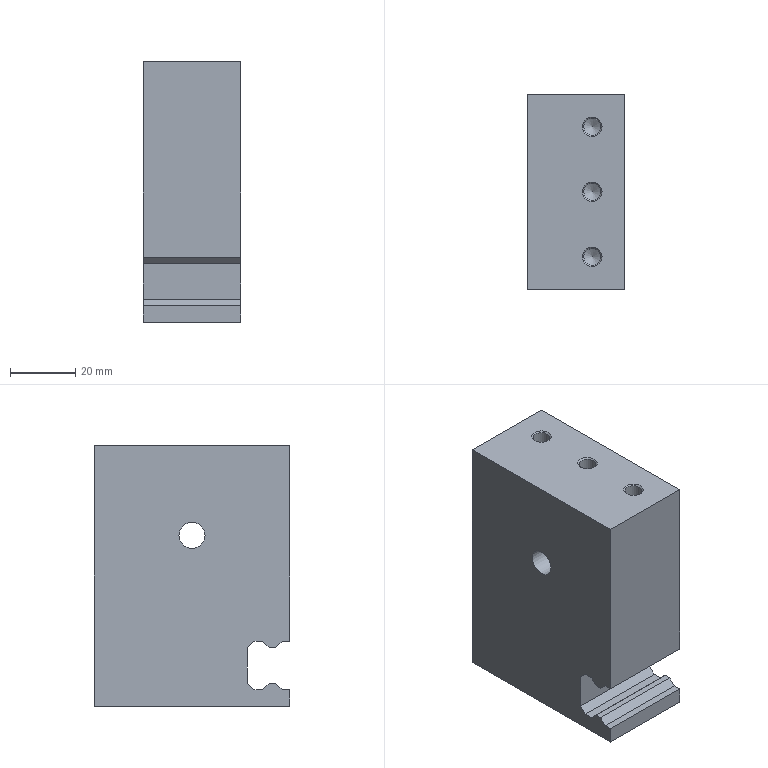Part | NX | features CBORE_HOLE 8, DATUM_CSYS 6, SYMBOLIC_THREAD 6, SIMPLE HOLE 5, SKETCH 5, HOLE PACKAGE 3, EXTRUDE 2, SUBTRACT 1 | 1 solid | 36 faces | box 30 x 60 x 80 mm | volume 135184 mm3 | plane 20 | cone 10 | cylinder 6 | commonest cylinder face diameters 5.2 x5 8 x1
STEP:
#1=CARTESIAN_POINT('',(15.,-2.3,7.5));
#2=VERTEX_POINT('',#1);
#3=CARTESIAN_POINT('',(-15.,-2.3,7.5));
#4=VERTEX_POINT('',#3);
#5=CARTESIAN_POINT('',(15.,-2.3,7.5));
#6=DIRECTION('',(-1.,0.,0.));
#7=VECTOR('',#6,1000.);
#8=LINE('',#5,#7);
#9=EDGE_CURVE('',#2,#4,#8,.T.);
#10=ORIENTED_EDGE('',*,*,#9,.F.);
#11=CARTESIAN_POINT('',(15.,-2.3,67.5));
#12=VERTEX_POINT('',#11);
#13=CARTESIAN_POINT('',(15.,-2.3,67.5));
#14=DIRECTION('',(0.,0.,-1.));
#15=VECTOR('',#14,1000.);
#16=LINE('',#13,#15);
#17=EDGE_CURVE('',#12,#2,#16,.T.);
#18=ORIENTED_EDGE('',*,*,#17,.F.);
#19=CARTESIAN_POINT('',(-15.,-2.3,67.5));
#20=VERTEX_POINT('',#19);
#21=CARTESIAN_POINT('',(15.,-2.3,67.5));
#22=DIRECTION('',(-1.,0.,0.));
#23=VECTOR('',#22,1000.);
#24=LINE('',#21,#23);
#25=EDGE_CURVE('',#12,#20,#24,.T.);
#26=ORIENTED_EDGE('',*,*,#25,.T.);
#27=CARTESIAN_POINT('',(-15.,-2.3,67.5));
#28=DIRECTION('',(0.,0.,-1.));
#29=VECTOR('',#28,1000.);
#30=LINE('',#27,#29);
#31=EDGE_CURVE('',#20,#4,#30,.T.);
#32=ORIENTED_EDGE('',*,*,#31,.T.);
#33=EDGE_LOOP('',(#10,#18,#26,#32));
#34=FACE_BOUND('',#33,.T.);
#35=CARTESIAN_POINT('',(15.,-2.3,67.5));
#36=DIRECTION('',(0.,1.,0.));
#37=DIRECTION('',(0.,0.,1.));
#38=AXIS2_PLACEMENT_3D('',#35,#36,#37);
#39=PLANE('',#38);
#40=ADVANCED_FACE('',(#34),#39,.F.);
#41=CARTESIAN_POINT('',(-15.,-2.3,-7.5));
#42=VERTEX_POINT('',#41);
#43=CARTESIAN_POINT('',(15.,-2.3,-7.5));
#44=VERTEX_POINT('',#43);
#45=CARTESIAN_POINT('',(15.,-2.3,-7.5));
#46=DIRECTION('',(1.,0.,0.));
#47=VECTOR('',#46,1000.);
#48=LINE('',#45,#47);
#49=EDGE_CURVE('',#42,#44,#48,.T.);
#50=ORIENTED_EDGE('',*,*,#49,.F.);
#51=CARTESIAN_POINT('',(-15.,-2.3,-12.5));
#52=VERTEX_POINT('',#51);
#53=CARTESIAN_POINT('',(-15.,-2.3,67.5));
#54=DIRECTION('',(0.,0.,-1.));
#55=VECTOR('',#54,1000.);
#56=LINE('',#53,#55);
#57=EDGE_CURVE('',#42,#52,#56,.T.);
#58=ORIENTED_EDGE('',*,*,#57,.T.);
#59=CARTESIAN_POINT('',(15.,-2.3,-12.5));
#60=VERTEX_POINT('',#59);
#61=CARTESIAN_POINT('',(15.,-2.3,-12.5));
#62=DIRECTION('',(-1.,0.,0.));
#63=VECTOR('',#62,1000.);
#64=LINE('',#61,#63);
#65=EDGE_CURVE('',#60,#52,#64,.T.);
#66=ORIENTED_EDGE('',*,*,#65,.F.);
#67=CARTESIAN_POINT('',(15.,-2.3,67.5));
#68=DIRECTION('',(0.,0.,-1.));
#69=VECTOR('',#68,1000.);
#70=LINE('',#67,#69);
#71=EDGE_CURVE('',#44,#60,#70,.T.);
#72=ORIENTED_EDGE('',*,*,#71,.F.);
#73=EDGE_LOOP('',(#50,#58,#66,#72));
#74=FACE_BOUND('',#73,.T.);
#75=CARTESIAN_POINT('',(15.,-2.3,67.5));
#76=DIRECTION('',(0.,1.,0.));
#77=DIRECTION('',(0.,0.,1.));
#78=AXIS2_PLACEMENT_3D('',#75,#76,#77);
#79=PLANE('',#78);
#80=ADVANCED_FACE('',(#74),#79,.F.);
#81=CARTESIAN_POINT('',(15.,31.7,40.));
#82=VERTEX_POINT('',#81);
#83=CARTESIAN_POINT('',(15.,27.7,40.));
#84=DIRECTION('',(1.,0.,0.));
#85=DIRECTION('',(0.,1.,0.));
#86=AXIS2_PLACEMENT_3D('',#83,#84,#85);
#87=CIRCLE('',#86,4.);
#88=EDGE_CURVE('',#82,#82,#87,.T.);
#89=ORIENTED_EDGE('',*,*,#88,.F.);
#90=EDGE_LOOP('',(#89));
#91=FACE_BOUND('',#90,.T.);
#92=ORIENTED_EDGE('',*,*,#17,.T.);
#93=CARTESIAN_POINT('',(15.,0.,7.5));
#94=VERTEX_POINT('',#93);
#95=CARTESIAN_POINT('',(15.,27.7,7.5));
#96=DIRECTION('',(0.,1.,0.));
#97=VECTOR('',#96,1000.);
#98=LINE('',#95,#97);
#99=EDGE_CURVE('',#2,#94,#98,.T.);
#100=ORIENTED_EDGE('',*,*,#99,.T.);
#101=CARTESIAN_POINT('',(15.,2.,5.5));
#102=VERTEX_POINT('',#101);
#103=CARTESIAN_POINT('',(15.,-2.4,9.9));
#104=DIRECTION('',(0.,0.7071,-0.7071));
#105=VECTOR('',#104,1000.);
#106=LINE('',#103,#105);
#107=EDGE_CURVE('',#94,#102,#106,.T.);
#108=ORIENTED_EDGE('',*,*,#107,.T.);
#109=CARTESIAN_POINT('',(15.,4.,5.5));
#110=VERTEX_POINT('',#109);
#111=CARTESIAN_POINT('',(15.,27.7,5.5));
#112=DIRECTION('',(0.,1.,0.));
#113=VECTOR('',#112,1000.);
#114=LINE('',#111,#113);
#115=EDGE_CURVE('',#102,#110,#114,.T.);
#116=ORIENTED_EDGE('',*,*,#115,.T.);
#117=CARTESIAN_POINT('',(15.,6.,7.5));
#118=VERTEX_POINT('',#117);
#119=CARTESIAN_POINT('',(15.,33.1,34.6));
#120=DIRECTION('',(0.,0.7071,0.7071));
#121=VECTOR('',#120,1000.);
#122=LINE('',#119,#121);
#123=EDGE_CURVE('',#110,#118,#122,.T.);
#124=ORIENTED_EDGE('',*,*,#123,.T.);
#125=CARTESIAN_POINT('',(15.,8.7,7.5));
#126=VERTEX_POINT('',#125);
#127=CARTESIAN_POINT('',(15.,27.7,7.5));
#128=DIRECTION('',(0.,1.,0.));
#129=VECTOR('',#128,1000.);
#130=LINE('',#127,#129);
#131=EDGE_CURVE('',#118,#126,#130,.T.);
#132=ORIENTED_EDGE('',*,*,#131,.T.);
#133=CARTESIAN_POINT('',(15.,10.7,5.5));
#134=VERTEX_POINT('',#133);
#135=CARTESIAN_POINT('',(15.,1.95,14.25));
#136=DIRECTION('',(0.,0.7071,-0.7071));
#137=VECTOR('',#136,1000.);
#138=LINE('',#135,#137);
#139=EDGE_CURVE('',#126,#134,#138,.T.);
#140=ORIENTED_EDGE('',*,*,#139,.T.);
#141=CARTESIAN_POINT('',(15.,10.7,-5.5));
#142=VERTEX_POINT('',#141);
#143=CARTESIAN_POINT('',(15.,10.7,40.));
#144=DIRECTION('',(0.,0.,-1.));
#145=VECTOR('',#144,1000.);
#146=LINE('',#143,#145);
#147=EDGE_CURVE('',#134,#142,#146,.T.);
#148=ORIENTED_EDGE('',*,*,#147,.T.);
#149=CARTESIAN_POINT('',(15.,8.7,-7.5));
#150=VERTEX_POINT('',#149);
#151=CARTESIAN_POINT('',(15.,41.95,25.75));
#152=DIRECTION('',(0.,-0.7071,-0.7071));
#153=VECTOR('',#152,1000.);
#154=LINE('',#151,#153);
#155=EDGE_CURVE('',#142,#150,#154,.T.);
#156=ORIENTED_EDGE('',*,*,#155,.T.);
#157=CARTESIAN_POINT('',(15.,6.,-7.5));
#158=VERTEX_POINT('',#157);
#159=CARTESIAN_POINT('',(15.,27.7,-7.5));
#160=DIRECTION('',(0.,-1.,0.));
#161=VECTOR('',#160,1000.);
#162=LINE('',#159,#161);
#163=EDGE_CURVE('',#150,#158,#162,.T.);
#164=ORIENTED_EDGE('',*,*,#163,.T.);
#165=CARTESIAN_POINT('',(15.,4.,-5.5));
#166=VERTEX_POINT('',#165);
#167=CARTESIAN_POINT('',(15.,-6.9,5.4));
#168=DIRECTION('',(0.,-0.7071,0.7071));
#169=VECTOR('',#168,1000.);
#170=LINE('',#167,#169);
#171=EDGE_CURVE('',#158,#166,#170,.T.);
#172=ORIENTED_EDGE('',*,*,#171,.T.);
#173=CARTESIAN_POINT('',(15.,2.,-5.5));
#174=VERTEX_POINT('',#173);
#175=CARTESIAN_POINT('',(15.,27.7,-5.5));
#176=DIRECTION('',(0.,-1.,0.));
#177=VECTOR('',#176,1000.);
#178=LINE('',#175,#177);
#179=EDGE_CURVE('',#166,#174,#178,.T.);
#180=ORIENTED_EDGE('',*,*,#179,.T.);
#181=CARTESIAN_POINT('',(15.,0.,-7.5));
#182=VERTEX_POINT('',#181);
#183=CARTESIAN_POINT('',(15.,37.6,30.1));
#184=DIRECTION('',(0.,-0.7071,-0.7071));
#185=VECTOR('',#184,1000.);
#186=LINE('',#183,#185);
#187=EDGE_CURVE('',#174,#182,#186,.T.);
#188=ORIENTED_EDGE('',*,*,#187,.T.);
#189=CARTESIAN_POINT('',(15.,27.7,-7.5));
#190=DIRECTION('',(0.,-1.,0.));
#191=VECTOR('',#190,1000.);
#192=LINE('',#189,#191);
#193=EDGE_CURVE('',#182,#44,#192,.T.);
#194=ORIENTED_EDGE('',*,*,#193,.T.);
#195=ORIENTED_EDGE('',*,*,#71,.T.);
#196=CARTESIAN_POINT('',(15.,57.7,-12.5));
#197=VERTEX_POINT('',#196);
#198=CARTESIAN_POINT('',(15.,-2.3,-12.5));
#199=DIRECTION('',(0.,1.,0.));
#200=VECTOR('',#199,1000.);
#201=LINE('',#198,#200);
#202=EDGE_CURVE('',#60,#197,#201,.T.);
#203=ORIENTED_EDGE('',*,*,#202,.T.);
#204=CARTESIAN_POINT('',(15.,57.7,67.5));
#205=VERTEX_POINT('',#204);
#206=CARTESIAN_POINT('',(15.,57.7,-12.5));
#207=DIRECTION('',(0.,0.,1.));
#208=VECTOR('',#207,1000.);
#209=LINE('',#206,#208);
#210=EDGE_CURVE('',#197,#205,#209,.T.);
#211=ORIENTED_EDGE('',*,*,#210,.T.);
#212=CARTESIAN_POINT('',(15.,57.7,67.5));
#213=DIRECTION('',(0.,-1.,0.));
#214=VECTOR('',#213,1000.);
#215=LINE('',#212,#214);
#216=EDGE_CURVE('',#205,#12,#215,.T.);
#217=ORIENTED_EDGE('',*,*,#216,.T.);
#218=EDGE_LOOP('',(#92,#100,#108,#116,#124,#132,#140,#148,#156,#164,#172,#180,#188,#194,#195,#203,#211,#217));
#219=FACE_BOUND('',#218,.T.);
#220=CARTESIAN_POINT('',(15.,27.7,40.));
#221=DIRECTION('',(1.,0.,0.));
#222=DIRECTION('',(0.,0.,-1.));
#223=AXIS2_PLACEMENT_3D('',#220,#221,#222);
#224=PLANE('',#223);
#225=ADVANCED_FACE('',(#91,#219),#224,.T.);
#226=CARTESIAN_POINT('',(-15.,31.7,40.));
#227=VERTEX_POINT('',#226);
#228=CARTESIAN_POINT('',(-15.,27.7,40.));
#229=DIRECTION('',(1.,0.,0.));
#230=DIRECTION('',(0.,1.,0.));
#231=AXIS2_PLACEMENT_3D('',#228,#229,#230);
#232=CIRCLE('',#231,4.);
#233=EDGE_CURVE('',#227,#227,#232,.T.);
#234=ORIENTED_EDGE('',*,*,#233,.T.);
#235=EDGE_LOOP('',(#234));
#236=FACE_BOUND('',#235,.T.);
#237=CARTESIAN_POINT('',(-15.,0.,7.5));
#238=VERTEX_POINT('',#237);
#239=CARTESIAN_POINT('',(-15.,27.7,7.5));
#240=DIRECTION('',(0.,1.,0.));
#241=VECTOR('',#240,1000.);
#242=LINE('',#239,#241);
#243=EDGE_CURVE('',#4,#238,#242,.T.);
#244=ORIENTED_EDGE('',*,*,#243,.F.);
#245=ORIENTED_EDGE('',*,*,#31,.F.);
#246=CARTESIAN_POINT('',(-15.,57.7,67.5));
#247=VERTEX_POINT('',#246);
#248=CARTESIAN_POINT('',(-15.,57.7,67.5));
#249=DIRECTION('',(0.,-1.,0.));
#250=VECTOR('',#249,1000.);
#251=LINE('',#248,#250);
#252=EDGE_CURVE('',#247,#20,#251,.T.);
#253=ORIENTED_EDGE('',*,*,#252,.F.);
#254=CARTESIAN_POINT('',(-15.,57.7,-12.5));
#255=VERTEX_POINT('',#254);
#256=CARTESIAN_POINT('',(-15.,57.7,-12.5));
#257=DIRECTION('',(0.,0.,1.));
#258=VECTOR('',#257,1000.);
#259=LINE('',#256,#258);
#260=EDGE_CURVE('',#255,#247,#259,.T.);
#261=ORIENTED_EDGE('',*,*,#260,.F.);
#262=CARTESIAN_POINT('',(-15.,-2.3,-12.5));
#263=DIRECTION('',(0.,1.,0.));
#264=VECTOR('',#263,1000.);
#265=LINE('',#262,#264);
#266=EDGE_CURVE('',#52,#255,#265,.T.);
#267=ORIENTED_EDGE('',*,*,#266,.F.);
#268=ORIENTED_EDGE('',*,*,#57,.F.);
#269=CARTESIAN_POINT('',(-15.,0.,-7.5));
#270=VERTEX_POINT('',#269);
#271=CARTESIAN_POINT('',(-15.,27.7,-7.5));
#272=DIRECTION('',(0.,-1.,0.));
#273=VECTOR('',#272,1000.);
#274=LINE('',#271,#273);
#275=EDGE_CURVE('',#270,#42,#274,.T.);
#276=ORIENTED_EDGE('',*,*,#275,.F.);
#277=CARTESIAN_POINT('',(-15.,2.,-5.5));
#278=VERTEX_POINT('',#277);
#279=CARTESIAN_POINT('',(-15.,37.6,30.1));
#280=DIRECTION('',(0.,-0.7071,-0.7071));
#281=VECTOR('',#280,1000.);
#282=LINE('',#279,#281);
#283=EDGE_CURVE('',#278,#270,#282,.T.);
#284=ORIENTED_EDGE('',*,*,#283,.F.);
#285=CARTESIAN_POINT('',(-15.,4.,-5.5));
#286=VERTEX_POINT('',#285);
#287=CARTESIAN_POINT('',(-15.,27.7,-5.5));
#288=DIRECTION('',(0.,-1.,0.));
#289=VECTOR('',#288,1000.);
#290=LINE('',#287,#289);
#291=EDGE_CURVE('',#286,#278,#290,.T.);
#292=ORIENTED_EDGE('',*,*,#291,.F.);
#293=CARTESIAN_POINT('',(-15.,6.,-7.5));
#294=VERTEX_POINT('',#293);
#295=CARTESIAN_POINT('',(-15.,-6.9,5.4));
#296=DIRECTION('',(0.,-0.7071,0.7071));
#297=VECTOR('',#296,1000.);
#298=LINE('',#295,#297);
#299=EDGE_CURVE('',#294,#286,#298,.T.);
#300=ORIENTED_EDGE('',*,*,#299,.F.);
#301=CARTESIAN_POINT('',(-15.,8.7,-7.5));
#302=VERTEX_POINT('',#301);
#303=CARTESIAN_POINT('',(-15.,27.7,-7.5));
#304=DIRECTION('',(0.,-1.,0.));
#305=VECTOR('',#304,1000.);
#306=LINE('',#303,#305);
#307=EDGE_CURVE('',#302,#294,#306,.T.);
#308=ORIENTED_EDGE('',*,*,#307,.F.);
#309=CARTESIAN_POINT('',(-15.,10.7,-5.5));
#310=VERTEX_POINT('',#309);
#311=CARTESIAN_POINT('',(-15.,41.95,25.75));
#312=DIRECTION('',(0.,-0.7071,-0.7071));
#313=VECTOR('',#312,1000.);
#314=LINE('',#311,#313);
#315=EDGE_CURVE('',#310,#302,#314,.T.);
#316=ORIENTED_EDGE('',*,*,#315,.F.);
#317=CARTESIAN_POINT('',(-15.,10.7,5.5));
#318=VERTEX_POINT('',#317);
#319=CARTESIAN_POINT('',(-15.,10.7,40.));
#320=DIRECTION('',(0.,0.,-1.));
#321=VECTOR('',#320,1000.);
#322=LINE('',#319,#321);
#323=EDGE_CURVE('',#318,#310,#322,.T.);
#324=ORIENTED_EDGE('',*,*,#323,.F.);
#325=CARTESIAN_POINT('',(-15.,8.7,7.5));
#326=VERTEX_POINT('',#325);
#327=CARTESIAN_POINT('',(-15.,1.95,14.25));
#328=DIRECTION('',(0.,0.7071,-0.7071));
#329=VECTOR('',#328,1000.);
#330=LINE('',#327,#329);
#331=EDGE_CURVE('',#326,#318,#330,.T.);
#332=ORIENTED_EDGE('',*,*,#331,.F.);
#333=CARTESIAN_POINT('',(-15.,6.,7.5));
#334=VERTEX_POINT('',#333);
#335=CARTESIAN_POINT('',(-15.,27.7,7.5));
#336=DIRECTION('',(0.,1.,0.));
#337=VECTOR('',#336,1000.);
#338=LINE('',#335,#337);
#339=EDGE_CURVE('',#334,#326,#338,.T.);
#340=ORIENTED_EDGE('',*,*,#339,.F.);
#341=CARTESIAN_POINT('',(-15.,4.,5.5));
#342=VERTEX_POINT('',#341);
#343=CARTESIAN_POINT('',(-15.,33.1,34.6));
#344=DIRECTION('',(0.,0.7071,0.7071));
#345=VECTOR('',#344,1000.);
#346=LINE('',#343,#345);
#347=EDGE_CURVE('',#342,#334,#346,.T.);
#348=ORIENTED_EDGE('',*,*,#347,.F.);
#349=CARTESIAN_POINT('',(-15.,2.,5.5));
#350=VERTEX_POINT('',#349);
#351=CARTESIAN_POINT('',(-15.,27.7,5.5));
#352=DIRECTION('',(0.,1.,0.));
#353=VECTOR('',#352,1000.);
#354=LINE('',#351,#353);
#355=EDGE_CURVE('',#350,#342,#354,.T.);
#356=ORIENTED_EDGE('',*,*,#355,.F.);
#357=CARTESIAN_POINT('',(-15.,-2.4,9.9));
#358=DIRECTION('',(0.,0.7071,-0.7071));
#359=VECTOR('',#358,1000.);
#360=LINE('',#357,#359);
#361=EDGE_CURVE('',#238,#350,#360,.T.);
#362=ORIENTED_EDGE('',*,*,#361,.F.);
#363=EDGE_LOOP('',(#244,#245,#253,#261,#267,#268,#276,#284,#292,#300,#308,#316,#324,#332,#340,#348,#356,#362));
#364=FACE_BOUND('',#363,.T.);
#365=CARTESIAN_POINT('',(-15.,27.7,40.));
#366=DIRECTION('',(1.,0.,0.));
#367=DIRECTION('',(0.,0.,-1.));
#368=AXIS2_PLACEMENT_3D('',#365,#366,#367);
#369=PLANE('',#368);
#370=ADVANCED_FACE('',(#236,#364),#369,.F.);
#371=CARTESIAN_POINT('',(5.,44.7,-12.5));
#372=VERTEX_POINT('',#371);
#373=CARTESIAN_POINT('',(5.,47.7,-12.5));
#374=DIRECTION('',(0.,0.,1.));
#375=DIRECTION('',(0.,-1.,0.));
#376=AXIS2_PLACEMENT_3D('',#373,#374,#375);
#377=CIRCLE('',#376,3.);
#378=EDGE_CURVE('',#372,#372,#377,.T.);
#379=ORIENTED_EDGE('',*,*,#378,.T.);
#380=EDGE_LOOP('',(#379));
#381=FACE_BOUND('',#380,.T.);
#382=CARTESIAN_POINT('',(5.,24.7,-12.5));
#383=VERTEX_POINT('',#382);
#384=CARTESIAN_POINT('',(5.,27.7,-12.5));
#385=DIRECTION('',(0.,0.,1.));
#386=DIRECTION('',(0.,-1.,0.));
#387=AXIS2_PLACEMENT_3D('',#384,#385,#386);
#388=CIRCLE('',#387,3.);
#389=EDGE_CURVE('',#383,#383,#388,.T.);
#390=ORIENTED_EDGE('',*,*,#389,.T.);
#391=EDGE_LOOP('',(#390));
#392=FACE_BOUND('',#391,.T.);
#393=ORIENTED_EDGE('',*,*,#266,.T.);
#394=CARTESIAN_POINT('',(15.,57.7,-12.5));
#395=DIRECTION('',(-1.,0.,0.));
#396=VECTOR('',#395,1000.);
#397=LINE('',#394,#396);
#398=EDGE_CURVE('',#197,#255,#397,.T.);
#399=ORIENTED_EDGE('',*,*,#398,.F.);
#400=ORIENTED_EDGE('',*,*,#202,.F.);
#401=ORIENTED_EDGE('',*,*,#65,.T.);
#402=EDGE_LOOP('',(#393,#399,#400,#401));
#403=FACE_BOUND('',#402,.T.);
#404=CARTESIAN_POINT('',(15.,-2.3,-12.5));
#405=DIRECTION('',(0.,0.,1.));
#406=DIRECTION('',(0.,-1.,0.));
#407=AXIS2_PLACEMENT_3D('',#404,#405,#406);
#408=PLANE('',#407);
#409=ADVANCED_FACE('',(#381,#392,#403),#408,.F.);
#410=ORIENTED_EDGE('',*,*,#260,.T.);
#411=CARTESIAN_POINT('',(15.,57.7,67.5));
#412=DIRECTION('',(-1.,0.,0.));
#413=VECTOR('',#412,1000.);
#414=LINE('',#411,#413);
#415=EDGE_CURVE('',#205,#247,#414,.T.);
#416=ORIENTED_EDGE('',*,*,#415,.F.);
#417=ORIENTED_EDGE('',*,*,#210,.F.);
#418=ORIENTED_EDGE('',*,*,#398,.T.);
#419=EDGE_LOOP('',(#410,#416,#417,#418));
#420=FACE_BOUND('',#419,.T.);
#421=CARTESIAN_POINT('',(15.,57.7,-12.5));
#422=DIRECTION('',(0.,-1.,0.));
#423=DIRECTION('',(0.,0.,-1.));
#424=AXIS2_PLACEMENT_3D('',#421,#422,#423);
#425=PLANE('',#424);
#426=ADVANCED_FACE('',(#420),#425,.F.);
#427=CARTESIAN_POINT('',(2.,7.7,67.5));
#428=VERTEX_POINT('',#427);
#429=CARTESIAN_POINT('',(5.,7.7,67.5));
#430=DIRECTION('',(0.,0.,-1.));
#431=DIRECTION('',(-1.,0.,0.));
#432=AXIS2_PLACEMENT_3D('',#429,#430,#431);
#433=CIRCLE('',#432,3.);
#434=EDGE_CURVE('',#428,#428,#433,.T.);
#435=ORIENTED_EDGE('',*,*,#434,.T.);
#436=EDGE_LOOP('',(#435));
#437=FACE_BOUND('',#436,.T.);
#438=CARTESIAN_POINT('',(2.,27.7,67.5));
#439=VERTEX_POINT('',#438);
#440=CARTESIAN_POINT('',(5.,27.7,67.5));
#441=DIRECTION('',(0.,0.,-1.));
#442=DIRECTION('',(-1.,0.,0.));
#443=AXIS2_PLACEMENT_3D('',#440,#441,#442);
#444=CIRCLE('',#443,3.);
#445=EDGE_CURVE('',#439,#439,#444,.T.);
#446=ORIENTED_EDGE('',*,*,#445,.T.);
#447=EDGE_LOOP('',(#446));
#448=FACE_BOUND('',#447,.T.);
#449=CARTESIAN_POINT('',(2.,47.7,67.5));
#450=VERTEX_POINT('',#449);
#451=CARTESIAN_POINT('',(5.,47.7,67.5));
#452=DIRECTION('',(0.,0.,-1.));
#453=DIRECTION('',(-1.,0.,0.));
#454=AXIS2_PLACEMENT_3D('',#451,#452,#453);
#455=CIRCLE('',#454,3.);
#456=EDGE_CURVE('',#450,#450,#455,.T.);
#457=ORIENTED_EDGE('',*,*,#456,.T.);
#458=EDGE_LOOP('',(#457));
#459=FACE_BOUND('',#458,.T.);
#460=ORIENTED_EDGE('',*,*,#252,.T.);
#461=ORIENTED_EDGE('',*,*,#25,.F.);
#462=ORIENTED_EDGE('',*,*,#216,.F.);
#463=ORIENTED_EDGE('',*,*,#415,.T.);
#464=EDGE_LOOP('',(#460,#461,#462,#463));
#465=FACE_BOUND('',#464,.T.);
#466=CARTESIAN_POINT('',(15.,57.7,67.5));
#467=DIRECTION('',(0.,0.,-1.));
#468=DIRECTION('',(-1.,0.,0.));
#469=AXIS2_PLACEMENT_3D('',#466,#467,#468);
#470=PLANE('',#469);
#471=ADVANCED_FACE('',(#437,#448,#459,#465),#470,.F.);
#472=ORIENTED_EDGE('',*,*,#88,.T.);
#473=EDGE_LOOP('',(#472));
#474=FACE_BOUND('',#473,.T.);
#475=ORIENTED_EDGE('',*,*,#233,.F.);
#476=EDGE_LOOP('',(#475));
#477=FACE_BOUND('',#476,.T.);
#478=CARTESIAN_POINT('',(15.,27.7,40.));
#479=DIRECTION('',(-1.,0.,0.));
#480=DIRECTION('',(0.,0.,1.));
#481=AXIS2_PLACEMENT_3D('',#478,#479,#480);
#482=CYLINDRICAL_SURFACE('',#481,4.);
#483=ADVANCED_FACE('',(#474,#477),#482,.F.);
#484=CARTESIAN_POINT('',(100.,2.,-5.5));
#485=DIRECTION('',(-1.,0.,0.));
#486=VECTOR('',#485,1000.);
#487=LINE('',#484,#486);
#488=EDGE_CURVE('',#278,#174,#487,.F.);
#489=ORIENTED_EDGE('',*,*,#488,.F.);
#490=ORIENTED_EDGE('',*,*,#283,.T.);
#491=CARTESIAN_POINT('',(100.,0.,-7.5));
#492=DIRECTION('',(-1.,0.,0.));
#493=VECTOR('',#492,1000.);
#494=LINE('',#491,#493);
#495=EDGE_CURVE('',#270,#182,#494,.F.);
#496=ORIENTED_EDGE('',*,*,#495,.T.);
#497=ORIENTED_EDGE('',*,*,#187,.F.);
#498=EDGE_LOOP('',(#489,#490,#496,#497));
#499=FACE_BOUND('',#498,.T.);
#500=CARTESIAN_POINT('',(100.,0.,-7.5));
#501=DIRECTION('',(0.,-0.7071,0.7071));
#502=DIRECTION('',(0.,-0.7071,-0.7071));
#503=AXIS2_PLACEMENT_3D('',#500,#501,#502);
#504=PLANE('',#503);
#505=ADVANCED_FACE('',(#499),#504,.T.);
#506=CARTESIAN_POINT('',(100.,4.,-5.5));
#507=DIRECTION('',(-1.,0.,0.));
#508=VECTOR('',#507,1000.);
#509=LINE('',#506,#508);
#510=EDGE_CURVE('',#286,#166,#509,.F.);
#511=ORIENTED_EDGE('',*,*,#510,.F.);
#512=ORIENTED_EDGE('',*,*,#291,.T.);
#513=ORIENTED_EDGE('',*,*,#488,.T.);
#514=ORIENTED_EDGE('',*,*,#179,.F.);
#515=EDGE_LOOP('',(#511,#512,#513,#514));
#516=FACE_BOUND('',#515,.T.);
#517=CARTESIAN_POINT('',(100.,2.,-5.5));
#518=DIRECTION('',(0.,0.,1.));
#519=DIRECTION('',(1.,0.,0.));
#520=AXIS2_PLACEMENT_3D('',#517,#518,#519);
#521=PLANE('',#520);
#522=ADVANCED_FACE('',(#516),#521,.T.);
#523=CARTESIAN_POINT('',(100.,6.,-7.5));
#524=DIRECTION('',(-1.,0.,0.));
#525=VECTOR('',#524,1000.);
#526=LINE('',#523,#525);
#527=EDGE_CURVE('',#294,#158,#526,.F.);
#528=ORIENTED_EDGE('',*,*,#527,.F.);
#529=ORIENTED_EDGE('',*,*,#299,.T.);
#530=ORIENTED_EDGE('',*,*,#510,.T.);
#531=ORIENTED_EDGE('',*,*,#171,.F.);
#532=EDGE_LOOP('',(#528,#529,#530,#531));
#533=FACE_BOUND('',#532,.T.);
#534=CARTESIAN_POINT('',(100.,4.,-5.5));
#535=DIRECTION('',(0.,0.7071,0.7071));
#536=DIRECTION('',(0.,-0.7071,0.7071));
#537=AXIS2_PLACEMENT_3D('',#534,#535,#536);
#538=PLANE('',#537);
#539=ADVANCED_FACE('',(#533),#538,.T.);
#540=CARTESIAN_POINT('',(100.,8.7,-7.5));
#541=DIRECTION('',(-1.,0.,0.));
#542=VECTOR('',#541,1000.);
#543=LINE('',#540,#542);
#544=EDGE_CURVE('',#302,#150,#543,.F.);
#545=ORIENTED_EDGE('',*,*,#544,.F.);
#546=ORIENTED_EDGE('',*,*,#307,.T.);
#547=ORIENTED_EDGE('',*,*,#527,.T.);
#548=ORIENTED_EDGE('',*,*,#163,.F.);
#549=EDGE_LOOP('',(#545,#546,#547,#548));
#550=FACE_BOUND('',#549,.T.);
#551=CARTESIAN_POINT('',(100.,6.,-7.5));
#552=DIRECTION('',(0.,0.,1.));
#553=DIRECTION('',(0.,-1.,0.));
#554=AXIS2_PLACEMENT_3D('',#551,#552,#553);
#555=PLANE('',#554);
#556=ADVANCED_FACE('',(#550),#555,.T.);
#557=CARTESIAN_POINT('',(100.,10.7,-5.5));
#558=DIRECTION('',(-1.,0.,0.));
#559=VECTOR('',#558,1000.);
#560=LINE('',#557,#559);
#561=EDGE_CURVE('',#310,#142,#560,.F.);
#562=ORIENTED_EDGE('',*,*,#561,.F.);
#563=ORIENTED_EDGE('',*,*,#315,.T.);
#564=ORIENTED_EDGE('',*,*,#544,.T.);
#565=ORIENTED_EDGE('',*,*,#155,.F.);
#566=EDGE_LOOP('',(#562,#563,#564,#565));
#567=FACE_BOUND('',#566,.T.);
#568=CARTESIAN_POINT('',(100.,8.7,-7.5));
#569=DIRECTION('',(0.,-0.7071,0.7071));
#570=DIRECTION('',(0.,-0.7071,-0.7071));
#571=AXIS2_PLACEMENT_3D('',#568,#569,#570);
#572=PLANE('',#571);
#573=ADVANCED_FACE('',(#567),#572,.T.);
#574=CARTESIAN_POINT('',(100.,10.7,5.5));
#575=DIRECTION('',(-1.,0.,0.));
#576=VECTOR('',#575,1000.);
#577=LINE('',#574,#576);
#578=EDGE_CURVE('',#318,#134,#577,.F.);
#579=ORIENTED_EDGE('',*,*,#578,.F.);
#580=ORIENTED_EDGE('',*,*,#323,.T.);
#581=ORIENTED_EDGE('',*,*,#561,.T.);
#582=ORIENTED_EDGE('',*,*,#147,.F.);
#583=EDGE_LOOP('',(#579,#580,#581,#582));
#584=FACE_BOUND('',#583,.T.);
#585=CARTESIAN_POINT('',(100.,10.7,0.));
#586=DIRECTION('',(0.,-1.,0.));
#587=DIRECTION('',(0.,0.,-1.));
#588=AXIS2_PLACEMENT_3D('',#585,#586,#587);
#589=PLANE('',#588);
#590=ADVANCED_FACE('',(#584),#589,.T.);
#591=CARTESIAN_POINT('',(100.,8.7,7.5));
#592=DIRECTION('',(-1.,0.,0.));
#593=VECTOR('',#592,1000.);
#594=LINE('',#591,#593);
#595=EDGE_CURVE('',#326,#126,#594,.F.);
#596=ORIENTED_EDGE('',*,*,#595,.F.);
#597=ORIENTED_EDGE('',*,*,#331,.T.);
#598=ORIENTED_EDGE('',*,*,#578,.T.);
#599=ORIENTED_EDGE('',*,*,#139,.F.);
#600=EDGE_LOOP('',(#596,#597,#598,#599));
#601=FACE_BOUND('',#600,.T.);
#602=CARTESIAN_POINT('',(100.,10.7,5.5));
#603=DIRECTION('',(0.,-0.7071,-0.7071));
#604=DIRECTION('',(0.,0.7071,-0.7071));
#605=AXIS2_PLACEMENT_3D('',#602,#603,#604);
#606=PLANE('',#605);
#607=ADVANCED_FACE('',(#601),#606,.T.);
#608=CARTESIAN_POINT('',(100.,6.,7.5));
#609=DIRECTION('',(-1.,0.,0.));
#610=VECTOR('',#609,1000.);
#611=LINE('',#608,#610);
#612=EDGE_CURVE('',#334,#118,#611,.F.);
#613=ORIENTED_EDGE('',*,*,#612,.F.);
#614=ORIENTED_EDGE('',*,*,#339,.T.);
#615=ORIENTED_EDGE('',*,*,#595,.T.);
#616=ORIENTED_EDGE('',*,*,#131,.F.);
#617=EDGE_LOOP('',(#613,#614,#615,#616));
#618=FACE_BOUND('',#617,.T.);
#619=CARTESIAN_POINT('',(100.,8.7,7.5));
#620=DIRECTION('',(0.,0.,-1.));
#621=DIRECTION('',(0.,1.,0.));
#622=AXIS2_PLACEMENT_3D('',#619,#620,#621);
#623=PLANE('',#622);
#624=ADVANCED_FACE('',(#618),#623,.T.);
#625=CARTESIAN_POINT('',(100.,4.,5.5));
#626=DIRECTION('',(-1.,0.,0.));
#627=VECTOR('',#626,1000.);
#628=LINE('',#625,#627);
#629=EDGE_CURVE('',#342,#110,#628,.F.);
#630=ORIENTED_EDGE('',*,*,#629,.F.);
#631=ORIENTED_EDGE('',*,*,#347,.T.);
#632=ORIENTED_EDGE('',*,*,#612,.T.);
#633=ORIENTED_EDGE('',*,*,#123,.F.);
#634=EDGE_LOOP('',(#630,#631,#632,#633));
#635=FACE_BOUND('',#634,.T.);
#636=CARTESIAN_POINT('',(100.,6.,7.5));
#637=DIRECTION('',(0.,0.7071,-0.7071));
#638=DIRECTION('',(0.,0.7071,0.7071));
#639=AXIS2_PLACEMENT_3D('',#636,#637,#638);
#640=PLANE('',#639);
#641=ADVANCED_FACE('',(#635),#640,.T.);
#642=CARTESIAN_POINT('',(100.,2.,5.5));
#643=DIRECTION('',(-1.,0.,0.));
#644=VECTOR('',#643,1000.);
#645=LINE('',#642,#644);
#646=EDGE_CURVE('',#350,#102,#645,.F.);
#647=ORIENTED_EDGE('',*,*,#646,.F.);
#648=ORIENTED_EDGE('',*,*,#355,.T.);
#649=ORIENTED_EDGE('',*,*,#629,.T.);
#650=ORIENTED_EDGE('',*,*,#115,.F.);
#651=EDGE_LOOP('',(#647,#648,#649,#650));
#652=FACE_BOUND('',#651,.T.);
#653=CARTESIAN_POINT('',(100.,4.,5.5));
#654=DIRECTION('',(0.,0.,-1.));
#655=DIRECTION('',(-1.,0.,0.));
#656=AXIS2_PLACEMENT_3D('',#653,#654,#655);
#657=PLANE('',#656);
#658=ADVANCED_FACE('',(#652),#657,.T.);
#659=CARTESIAN_POINT('',(100.,0.,7.5));
#660=DIRECTION('',(-1.,0.,0.));
#661=VECTOR('',#660,1000.);
#662=LINE('',#659,#661);
#663=EDGE_CURVE('',#238,#94,#662,.F.);
#664=ORIENTED_EDGE('',*,*,#663,.F.);
#665=ORIENTED_EDGE('',*,*,#361,.T.);
#666=ORIENTED_EDGE('',*,*,#646,.T.);
#667=ORIENTED_EDGE('',*,*,#107,.F.);
#668=EDGE_LOOP('',(#664,#665,#666,#667));
#669=FACE_BOUND('',#668,.T.);
#670=CARTESIAN_POINT('',(100.,2.,5.5));
#671=DIRECTION('',(0.,-0.7071,-0.7071));
#672=DIRECTION('',(0.,0.7071,-0.7071));
#673=AXIS2_PLACEMENT_3D('',#670,#671,#672);
#674=PLANE('',#673);
#675=ADVANCED_FACE('',(#669),#674,.T.);
#676=ORIENTED_EDGE('',*,*,#9,.T.);
#677=ORIENTED_EDGE('',*,*,#243,.T.);
#678=ORIENTED_EDGE('',*,*,#663,.T.);
#679=ORIENTED_EDGE('',*,*,#99,.F.);
#680=EDGE_LOOP('',(#676,#677,#678,#679));
#681=FACE_BOUND('',#680,.T.);
#682=CARTESIAN_POINT('',(100.,0.,7.5));
#683=DIRECTION('',(0.,0.,-1.));
#684=DIRECTION('',(0.,1.,0.));
#685=AXIS2_PLACEMENT_3D('',#682,#683,#684);
#686=PLANE('',#685);
#687=ADVANCED_FACE('',(#681),#686,.T.);
#688=ORIENTED_EDGE('',*,*,#495,.F.);
#689=ORIENTED_EDGE('',*,*,#275,.T.);
#690=ORIENTED_EDGE('',*,*,#49,.T.);
#691=ORIENTED_EDGE('',*,*,#193,.F.);
#692=EDGE_LOOP('',(#688,#689,#690,#691));
#693=FACE_BOUND('',#692,.T.);
#694=CARTESIAN_POINT('',(100.,-4.3,-7.5));
#695=DIRECTION('',(0.,0.,1.));
#696=DIRECTION('',(0.,-1.,0.));
#697=AXIS2_PLACEMENT_3D('',#694,#695,#696);
#698=PLANE('',#697);
#699=ADVANCED_FACE('',(#693),#698,.T.);
#700=CARTESIAN_POINT('',(2.4,47.7,49.5));
#701=VERTEX_POINT('',#700);
#702=CARTESIAN_POINT('',(5.,47.7,49.5));
#703=DIRECTION('',(0.,0.,-1.));
#704=DIRECTION('',(-1.,0.,0.));
#705=AXIS2_PLACEMENT_3D('',#702,#703,#704);
#706=CIRCLE('',#705,2.6);
#707=EDGE_CURVE('',#701,#701,#706,.F.);
#708=ORIENTED_EDGE('',*,*,#707,.T.);
#709=EDGE_LOOP('',(#708));
#710=FACE_BOUND('',#709,.T.);
#711=CARTESIAN_POINT('',(5.,47.7,47.938));
#712=VERTEX_POINT('',#711);
#713=VERTEX_LOOP('',#712);
#714=FACE_BOUND('',#713,.T.);
#715=CARTESIAN_POINT('',(5.,47.7,49.5));
#716=DIRECTION('',(0.,0.,1.));
#717=DIRECTION('',(1.,0.,0.));
#718=AXIS2_PLACEMENT_3D('',#715,#716,#717);
#719=CONICAL_SURFACE('',#718,2.6,1.03);
#720=ADVANCED_FACE('',(#710,#714),#719,.F.);
#721=CARTESIAN_POINT('',(2.4,47.7,67.1));
#722=VERTEX_POINT('',#721);
#723=CARTESIAN_POINT('',(5.,47.7,67.1));
#724=DIRECTION('',(0.,0.,-1.));
#725=DIRECTION('',(-1.,0.,0.));
#726=AXIS2_PLACEMENT_3D('',#723,#724,#725);
#727=CIRCLE('',#726,2.6);
#728=EDGE_CURVE('',#722,#722,#727,.F.);
#729=ORIENTED_EDGE('',*,*,#728,.T.);
#730=EDGE_LOOP('',(#729));
#731=FACE_BOUND('',#730,.T.);
#732=ORIENTED_EDGE('',*,*,#707,.F.);
#733=EDGE_LOOP('',(#732));
#734=FACE_BOUND('',#733,.T.);
#735=CARTESIAN_POINT('',(5.,47.7,67.5));
#736=DIRECTION('',(0.,0.,-1.));
#737=DIRECTION('',(-1.,0.,0.));
#738=AXIS2_PLACEMENT_3D('',#735,#736,#737);
#739=CYLINDRICAL_SURFACE('',#738,2.6);
#740=ADVANCED_FACE('',(#731,#734),#739,.F.);
#741=ORIENTED_EDGE('',*,*,#728,.F.);
#742=EDGE_LOOP('',(#741));
#743=FACE_BOUND('',#742,.T.);
#744=ORIENTED_EDGE('',*,*,#456,.F.);
#745=EDGE_LOOP('',(#744));
#746=FACE_BOUND('',#745,.T.);
#747=CARTESIAN_POINT('',(5.,47.7,67.5));
#748=DIRECTION('',(0.,0.,1.));
#749=DIRECTION('',(1.,0.,0.));
#750=AXIS2_PLACEMENT_3D('',#747,#748,#749);
#751=CONICAL_SURFACE('',#750,3.,0.7854);
#752=ADVANCED_FACE('',(#743,#746),#751,.F.);
#753=CARTESIAN_POINT('',(2.4,27.7,49.5));
#754=VERTEX_POINT('',#753);
#755=CARTESIAN_POINT('',(5.,27.7,49.5));
#756=DIRECTION('',(0.,0.,-1.));
#757=DIRECTION('',(-1.,0.,0.));
#758=AXIS2_PLACEMENT_3D('',#755,#756,#757);
#759=CIRCLE('',#758,2.6);
#760=EDGE_CURVE('',#754,#754,#759,.F.);
#761=ORIENTED_EDGE('',*,*,#760,.T.);
#762=EDGE_LOOP('',(#761));
#763=FACE_BOUND('',#762,.T.);
#764=CARTESIAN_POINT('',(5.,27.7,47.938));
#765=VERTEX_POINT('',#764);
#766=VERTEX_LOOP('',#765);
#767=FACE_BOUND('',#766,.T.);
#768=CARTESIAN_POINT('',(5.,27.7,49.5));
#769=DIRECTION('',(0.,0.,1.));
#770=DIRECTION('',(1.,0.,0.));
#771=AXIS2_PLACEMENT_3D('',#768,#769,#770);
#772=CONICAL_SURFACE('',#771,2.6,1.03);
#773=ADVANCED_FACE('',(#763,#767),#772,.F.);
#774=CARTESIAN_POINT('',(2.4,27.7,67.1));
#775=VERTEX_POINT('',#774);
#776=CARTESIAN_POINT('',(5.,27.7,67.1));
#777=DIRECTION('',(0.,0.,-1.));
#778=DIRECTION('',(-1.,0.,0.));
#779=AXIS2_PLACEMENT_3D('',#776,#777,#778);
#780=CIRCLE('',#779,2.6);
#781=EDGE_CURVE('',#775,#775,#780,.F.);
#782=ORIENTED_EDGE('',*,*,#781,.T.);
#783=EDGE_LOOP('',(#782));
#784=FACE_BOUND('',#783,.T.);
#785=ORIENTED_EDGE('',*,*,#760,.F.);
#786=EDGE_LOOP('',(#785));
#787=FACE_BOUND('',#786,.T.);
#788=CARTESIAN_POINT('',(5.,27.7,67.5));
#789=DIRECTION('',(0.,0.,-1.));
#790=DIRECTION('',(-1.,0.,0.));
#791=AXIS2_PLACEMENT_3D('',#788,#789,#790);
#792=CYLINDRICAL_SURFACE('',#791,2.6);
#793=ADVANCED_FACE('',(#784,#787),#792,.F.);
#794=ORIENTED_EDGE('',*,*,#781,.F.);
#795=EDGE_LOOP('',(#794));
#796=FACE_BOUND('',#795,.T.);
#797=ORIENTED_EDGE('',*,*,#445,.F.);
#798=EDGE_LOOP('',(#797));
#799=FACE_BOUND('',#798,.T.);
#800=CARTESIAN_POINT('',(5.,27.7,67.5));
#801=DIRECTION('',(0.,0.,1.));
#802=DIRECTION('',(1.,0.,0.));
#803=AXIS2_PLACEMENT_3D('',#800,#801,#802);
#804=CONICAL_SURFACE('',#803,3.,0.7854);
#805=ADVANCED_FACE('',(#796,#799),#804,.F.);
#806=CARTESIAN_POINT('',(2.4,7.7,49.5));
#807=VERTEX_POINT('',#806);
#808=CARTESIAN_POINT('',(5.,7.7,49.5));
#809=DIRECTION('',(0.,0.,-1.));
#810=DIRECTION('',(-1.,0.,0.));
#811=AXIS2_PLACEMENT_3D('',#808,#809,#810);
#812=CIRCLE('',#811,2.6);
#813=EDGE_CURVE('',#807,#807,#812,.F.);
#814=ORIENTED_EDGE('',*,*,#813,.T.);
#815=EDGE_LOOP('',(#814));
#816=FACE_BOUND('',#815,.T.);
#817=CARTESIAN_POINT('',(5.,7.7,47.938));
#818=VERTEX_POINT('',#817);
#819=VERTEX_LOOP('',#818);
#820=FACE_BOUND('',#819,.T.);
#821=CARTESIAN_POINT('',(5.,7.7,49.5));
#822=DIRECTION('',(0.,0.,1.));
#823=DIRECTION('',(1.,0.,0.));
#824=AXIS2_PLACEMENT_3D('',#821,#822,#823);
#825=CONICAL_SURFACE('',#824,2.6,1.03);
#826=ADVANCED_FACE('',(#816,#820),#825,.F.);
#827=CARTESIAN_POINT('',(2.4,7.7,67.1));
#828=VERTEX_POINT('',#827);
#829=CARTESIAN_POINT('',(5.,7.7,67.1));
#830=DIRECTION('',(0.,0.,-1.));
#831=DIRECTION('',(-1.,0.,0.));
#832=AXIS2_PLACEMENT_3D('',#829,#830,#831);
#833=CIRCLE('',#832,2.6);
#834=EDGE_CURVE('',#828,#828,#833,.F.);
#835=ORIENTED_EDGE('',*,*,#834,.T.);
#836=EDGE_LOOP('',(#835));
#837=FACE_BOUND('',#836,.T.);
#838=ORIENTED_EDGE('',*,*,#813,.F.);
#839=EDGE_LOOP('',(#838));
#840=FACE_BOUND('',#839,.T.);
#841=CARTESIAN_POINT('',(5.,7.7,67.5));
#842=DIRECTION('',(0.,0.,-1.));
#843=DIRECTION('',(-1.,0.,0.));
#844=AXIS2_PLACEMENT_3D('',#841,#842,#843);
#845=CYLINDRICAL_SURFACE('',#844,2.6);
#846=ADVANCED_FACE('',(#837,#840),#845,.F.);
#847=ORIENTED_EDGE('',*,*,#834,.F.);
#848=EDGE_LOOP('',(#847));
#849=FACE_BOUND('',#848,.T.);
#850=ORIENTED_EDGE('',*,*,#434,.F.);
#851=EDGE_LOOP('',(#850));
#852=FACE_BOUND('',#851,.T.);
#853=CARTESIAN_POINT('',(5.,7.7,67.5));
#854=DIRECTION('',(0.,0.,1.));
#855=DIRECTION('',(1.,0.,0.));
#856=AXIS2_PLACEMENT_3D('',#853,#854,#855);
#857=CONICAL_SURFACE('',#856,3.,0.7854);
#858=ADVANCED_FACE('',(#849,#852),#857,.F.);
#859=CARTESIAN_POINT('',(5.,25.1,7.5));
#860=VERTEX_POINT('',#859);
#861=CARTESIAN_POINT('',(5.,27.7,7.5));
#862=DIRECTION('',(0.,0.,1.));
#863=DIRECTION('',(0.,-1.,0.));
#864=AXIS2_PLACEMENT_3D('',#861,#862,#863);
#865=CIRCLE('',#864,2.6);
#866=EDGE_CURVE('',#860,#860,#865,.F.);
#867=ORIENTED_EDGE('',*,*,#866,.T.);
#868=EDGE_LOOP('',(#867));
#869=FACE_BOUND('',#868,.T.);
#870=CARTESIAN_POINT('',(5.,27.7,9.062));
#871=VERTEX_POINT('',#870);
#872=VERTEX_LOOP('',#871);
#873=FACE_BOUND('',#872,.T.);
#874=CARTESIAN_POINT('',(5.,27.7,7.5));
#875=DIRECTION('',(0.,0.,-1.));
#876=DIRECTION('',(0.,1.,0.));
#877=AXIS2_PLACEMENT_3D('',#874,#875,#876);
#878=CONICAL_SURFACE('',#877,2.6,1.03);
#879=ADVANCED_FACE('',(#869,#873),#878,.F.);
#880=CARTESIAN_POINT('',(7.6,27.7,-12.1));
#881=VERTEX_POINT('',#880);
#882=CARTESIAN_POINT('',(5.,27.7,-12.1));
#883=DIRECTION('',(0.,0.,1.));
#884=DIRECTION('',(1.,0.,0.));
#885=AXIS2_PLACEMENT_3D('',#882,#883,#884);
#886=CIRCLE('',#885,2.6);
#887=EDGE_CURVE('',#881,#881,#886,.F.);
#888=ORIENTED_EDGE('',*,*,#887,.T.);
#889=EDGE_LOOP('',(#888));
#890=FACE_BOUND('',#889,.T.);
#891=ORIENTED_EDGE('',*,*,#866,.F.);
#892=EDGE_LOOP('',(#891));
#893=FACE_BOUND('',#892,.T.);
#894=CARTESIAN_POINT('',(5.,27.7,-12.5));
#895=DIRECTION('',(0.,0.,1.));
#896=DIRECTION('',(0.,-1.,0.));
#897=AXIS2_PLACEMENT_3D('',#894,#895,#896);
#898=CYLINDRICAL_SURFACE('',#897,2.6);
#899=ADVANCED_FACE('',(#890,#893),#898,.F.);
#900=ORIENTED_EDGE('',*,*,#887,.F.);
#901=EDGE_LOOP('',(#900));
#902=FACE_BOUND('',#901,.T.);
#903=ORIENTED_EDGE('',*,*,#389,.F.);
#904=EDGE_LOOP('',(#903));
#905=FACE_BOUND('',#904,.T.);
#906=CARTESIAN_POINT('',(5.,27.7,-12.5));
#907=DIRECTION('',(0.,0.,-1.));
#908=DIRECTION('',(-1.,0.,0.));
#909=AXIS2_PLACEMENT_3D('',#906,#907,#908);
#910=CONICAL_SURFACE('',#909,3.,0.7854);
#911=ADVANCED_FACE('',(#902,#905),#910,.F.);
#912=CARTESIAN_POINT('',(5.,45.1,7.5));
#913=VERTEX_POINT('',#912);
#914=CARTESIAN_POINT('',(5.,47.7,7.5));
#915=DIRECTION('',(0.,0.,1.));
#916=DIRECTION('',(0.,-1.,0.));
#917=AXIS2_PLACEMENT_3D('',#914,#915,#916);
#918=CIRCLE('',#917,2.6);
#919=EDGE_CURVE('',#913,#913,#918,.F.);
#920=ORIENTED_EDGE('',*,*,#919,.T.);
#921=EDGE_LOOP('',(#920));
#922=FACE_BOUND('',#921,.T.);
#923=CARTESIAN_POINT('',(5.,47.7,9.062));
#924=VERTEX_POINT('',#923);
#925=VERTEX_LOOP('',#924);
#926=FACE_BOUND('',#925,.T.);
#927=CARTESIAN_POINT('',(5.,47.7,7.5));
#928=DIRECTION('',(0.,0.,-1.));
#929=DIRECTION('',(0.,1.,0.));
#930=AXIS2_PLACEMENT_3D('',#927,#928,#929);
#931=CONICAL_SURFACE('',#930,2.6,1.03);
#932=ADVANCED_FACE('',(#922,#926),#931,.F.);
#933=CARTESIAN_POINT('',(7.6,47.7,-12.1));
#934=VERTEX_POINT('',#933);
#935=CARTESIAN_POINT('',(5.,47.7,-12.1));
#936=DIRECTION('',(0.,0.,1.));
#937=DIRECTION('',(1.,0.,0.));
#938=AXIS2_PLACEMENT_3D('',#935,#936,#937);
#939=CIRCLE('',#938,2.6);
#940=EDGE_CURVE('',#934,#934,#939,.F.);
#941=ORIENTED_EDGE('',*,*,#940,.T.);
#942=EDGE_LOOP('',(#941));
#943=FACE_BOUND('',#942,.T.);
#944=ORIENTED_EDGE('',*,*,#919,.F.);
#945=EDGE_LOOP('',(#944));
#946=FACE_BOUND('',#945,.T.);
#947=CARTESIAN_POINT('',(5.,47.7,-12.5));
#948=DIRECTION('',(0.,0.,1.));
#949=DIRECTION('',(0.,-1.,0.));
#950=AXIS2_PLACEMENT_3D('',#947,#948,#949);
#951=CYLINDRICAL_SURFACE('',#950,2.6);
#952=ADVANCED_FACE('',(#943,#946),#951,.F.);
#953=ORIENTED_EDGE('',*,*,#940,.F.);
#954=EDGE_LOOP('',(#953));
#955=FACE_BOUND('',#954,.T.);
#956=ORIENTED_EDGE('',*,*,#378,.F.);
#957=EDGE_LOOP('',(#956));
#958=FACE_BOUND('',#957,.T.);
#959=CARTESIAN_POINT('',(5.,47.7,-12.5));
#960=DIRECTION('',(0.,0.,-1.));
#961=DIRECTION('',(-1.,0.,0.));
#962=AXIS2_PLACEMENT_3D('',#959,#960,#961);
#963=CONICAL_SURFACE('',#962,3.,0.7854);
#964=ADVANCED_FACE('',(#955,#958),#963,.F.);
#965=CLOSED_SHELL('',(#40,#80,#225,#370,#409,#426,#471,#483,#505,#522,#539,#556,#573,#590,#607,#624,#641,#658,#675,#687,#699,#720,#740,#752,#773,#793,#805,#826,#846,#858,#879,#899,#911,#932,#952,#964));
#966=MANIFOLD_SOLID_BREP('',#965);
#967=(LENGTH_UNIT()NAMED_UNIT(*)SI_UNIT(.MILLI.,.METRE.));
#968=UNCERTAINTY_MEASURE_WITH_UNIT(LENGTH_MEASURE(0.00001),#967,'','');
#969=(NAMED_UNIT(*)PLANE_ANGLE_UNIT()SI_UNIT($,.RADIAN.));
#970=(NAMED_UNIT(*)SI_UNIT($,.STERADIAN.)SOLID_ANGLE_UNIT());
#971=(GEOMETRIC_REPRESENTATION_CONTEXT(3)GLOBAL_UNCERTAINTY_ASSIGNED_CONTEXT((#968))GLOBAL_UNIT_ASSIGNED_CONTEXT((#967,#969,#970))REPRESENTATION_CONTEXT('',''));
#972=ADVANCED_BREP_SHAPE_REPRESENTATION('',(#966),#971);